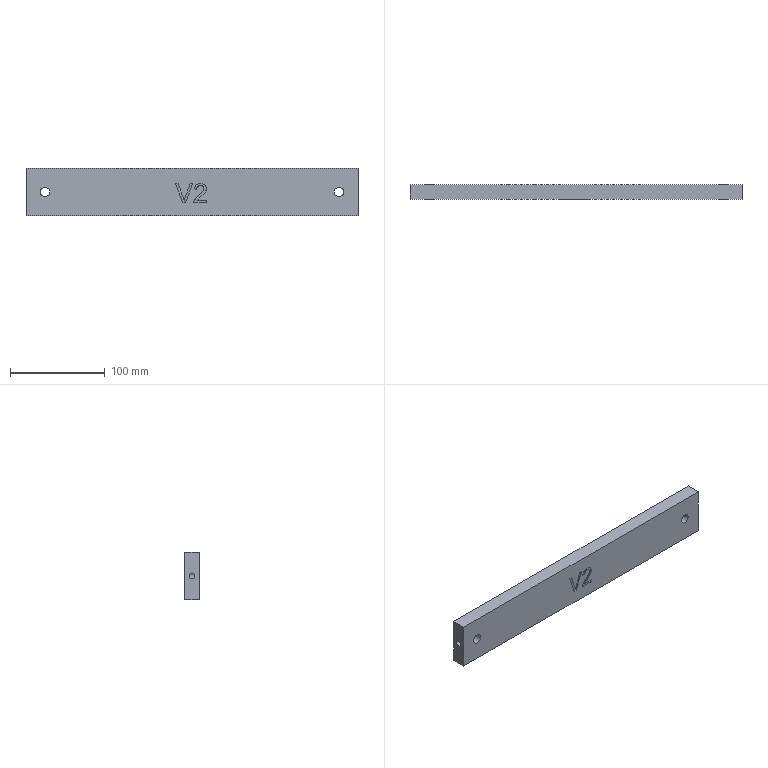Part | STEP file | Substructure | 1 solid | 43 faces | box 350 x 15 x 50 mm | volume 259181 mm3 | other 20 | plane 19 | cylinder 4 | commonest cylinder face diameters 6 x2 10 x2